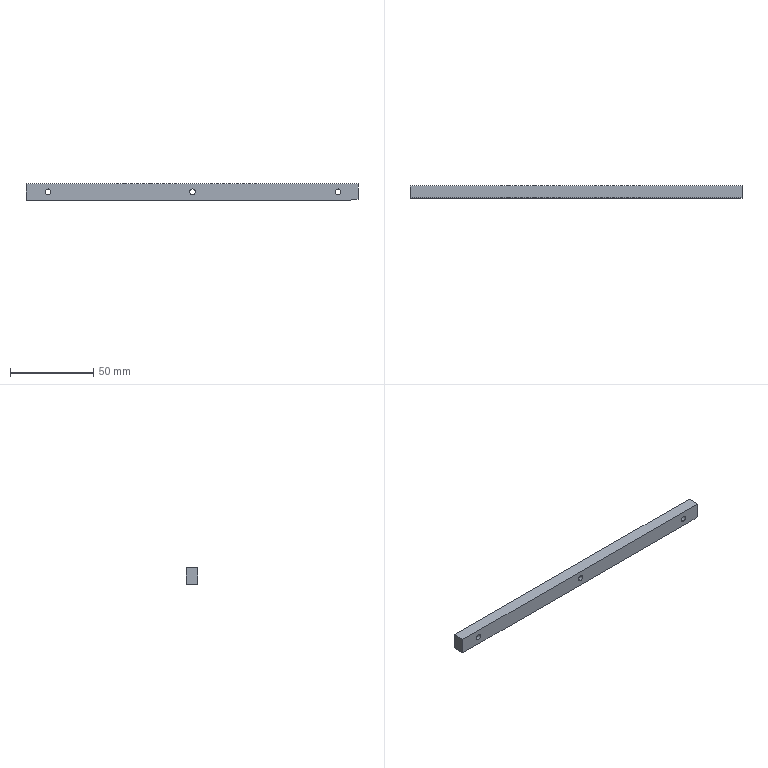Part | NX | 1 solid | 22 faces | box 199.5 x 7.2 x 9.8 mm | volume 13598 mm3 | cylinder 12 | plane 10 | commonest cylinder face diameters 3.5 x6 6 x6
STEP:
#1=CARTESIAN_POINT('',(659.5,215.9,-18.4));
#2=VERTEX_POINT('',#1);
#3=CARTESIAN_POINT('',(659.5,215.9,-27.763));
#4=VERTEX_POINT('',#3);
#5=CARTESIAN_POINT('',(659.5,215.9,-24.851));
#6=DIRECTION('',(0.,0.,-1.));
#7=VECTOR('',#6,1000.);
#8=LINE('',#5,#7);
#9=EDGE_CURVE('',#2,#4,#8,.T.);
#10=ORIENTED_EDGE('',*,*,#9,.T.);
#11=CARTESIAN_POINT('',(654.5,215.9,-28.2));
#12=VERTEX_POINT('',#11);
#13=CARTESIAN_POINT('',(660.,215.9,-27.719));
#14=DIRECTION('',(-0.9962,0.,-0.08716));
#15=VECTOR('',#14,1000.);
#16=LINE('',#13,#15);
#17=EDGE_CURVE('',#4,#12,#16,.T.);
#18=ORIENTED_EDGE('',*,*,#17,.T.);
#19=CARTESIAN_POINT('',(460.,215.9,-28.2));
#20=VERTEX_POINT('',#19);
#21=CARTESIAN_POINT('',(660.,215.9,-28.2));
#22=DIRECTION('',(1.,0.,0.));
#23=VECTOR('',#22,1000.);
#24=LINE('',#21,#23);
#25=EDGE_CURVE('',#20,#12,#24,.T.);
#26=ORIENTED_EDGE('',*,*,#25,.F.);
#27=CARTESIAN_POINT('',(460.,215.9,-18.4));
#28=VERTEX_POINT('',#27);
#29=CARTESIAN_POINT('',(460.,215.9,-24.851));
#30=DIRECTION('',(0.,0.,1.));
#31=VECTOR('',#30,1000.);
#32=LINE('',#29,#31);
#33=EDGE_CURVE('',#20,#28,#32,.T.);
#34=ORIENTED_EDGE('',*,*,#33,.T.);
#35=CARTESIAN_POINT('',(660.,215.9,-18.4));
#36=DIRECTION('',(1.,0.,0.));
#37=VECTOR('',#36,1000.);
#38=LINE('',#35,#37);
#39=EDGE_CURVE('',#28,#2,#38,.T.);
#40=ORIENTED_EDGE('',*,*,#39,.T.);
#41=EDGE_LOOP('',(#10,#18,#26,#34,#40));
#42=FACE_BOUND('',#41,.T.);
#43=CARTESIAN_POINT('',(647.5,215.9,-20.2));
#44=VERTEX_POINT('',#43);
#45=CARTESIAN_POINT('',(647.5,215.9,-26.2));
#46=VERTEX_POINT('',#45);
#47=CARTESIAN_POINT('',(647.5,215.9,-23.2));
#48=DIRECTION('',(0.,1.,0.));
#49=DIRECTION('',(0.,0.,-1.));
#50=AXIS2_PLACEMENT_3D('',#47,#48,#49);
#51=CIRCLE('',#50,3.);
#52=EDGE_CURVE('',#44,#46,#51,.T.);
#53=ORIENTED_EDGE('',*,*,#52,.F.);
#54=CARTESIAN_POINT('',(647.5,215.9,-23.2));
#55=DIRECTION('',(0.,1.,0.));
#56=DIRECTION('',(0.,0.,-1.));
#57=AXIS2_PLACEMENT_3D('',#54,#55,#56);
#58=CIRCLE('',#57,3.);
#59=EDGE_CURVE('',#46,#44,#58,.T.);
#60=ORIENTED_EDGE('',*,*,#59,.F.);
#61=EDGE_LOOP('',(#53,#60));
#62=FACE_BOUND('',#61,.T.);
#63=CARTESIAN_POINT('',(560.,215.9,-20.2));
#64=VERTEX_POINT('',#63);
#65=CARTESIAN_POINT('',(560.,215.9,-26.2));
#66=VERTEX_POINT('',#65);
#67=CARTESIAN_POINT('',(560.,215.9,-23.2));
#68=DIRECTION('',(0.,1.,0.));
#69=DIRECTION('',(0.,0.,-1.));
#70=AXIS2_PLACEMENT_3D('',#67,#68,#69);
#71=CIRCLE('',#70,3.);
#72=EDGE_CURVE('',#64,#66,#71,.T.);
#73=ORIENTED_EDGE('',*,*,#72,.F.);
#74=CARTESIAN_POINT('',(560.,215.9,-23.2));
#75=DIRECTION('',(0.,1.,0.));
#76=DIRECTION('',(0.,0.,-1.));
#77=AXIS2_PLACEMENT_3D('',#74,#75,#76);
#78=CIRCLE('',#77,3.);
#79=EDGE_CURVE('',#66,#64,#78,.T.);
#80=ORIENTED_EDGE('',*,*,#79,.F.);
#81=EDGE_LOOP('',(#73,#80));
#82=FACE_BOUND('',#81,.T.);
#83=CARTESIAN_POINT('',(473.248,215.9,-20.2));
#84=VERTEX_POINT('',#83);
#85=CARTESIAN_POINT('',(473.248,215.9,-26.2));
#86=VERTEX_POINT('',#85);
#87=CARTESIAN_POINT('',(473.248,215.9,-23.2));
#88=DIRECTION('',(0.,1.,0.));
#89=DIRECTION('',(0.,0.,-1.));
#90=AXIS2_PLACEMENT_3D('',#87,#88,#89);
#91=CIRCLE('',#90,3.);
#92=EDGE_CURVE('',#84,#86,#91,.T.);
#93=ORIENTED_EDGE('',*,*,#92,.F.);
#94=CARTESIAN_POINT('',(473.248,215.9,-23.2));
#95=DIRECTION('',(0.,1.,0.));
#96=DIRECTION('',(0.,0.,-1.));
#97=AXIS2_PLACEMENT_3D('',#94,#95,#96);
#98=CIRCLE('',#97,3.);
#99=EDGE_CURVE('',#86,#84,#98,.T.);
#100=ORIENTED_EDGE('',*,*,#99,.F.);
#101=EDGE_LOOP('',(#93,#100));
#102=FACE_BOUND('',#101,.T.);
#103=CARTESIAN_POINT('',(660.,215.9,-28.2));
#104=DIRECTION('',(0.,1.,0.));
#105=DIRECTION('',(1.,0.,0.));
#106=AXIS2_PLACEMENT_3D('',#103,#104,#105);
#107=PLANE('',#106);
#108=ADVANCED_FACE('',(#42,#62,#82,#102),#107,.T.);
#109=CARTESIAN_POINT('',(654.5,208.7,-28.2));
#110=VERTEX_POINT('',#109);
#111=CARTESIAN_POINT('',(654.5,212.3,-28.2));
#112=DIRECTION('',(0.,-1.,0.));
#113=VECTOR('',#112,1000.);
#114=LINE('',#111,#113);
#115=EDGE_CURVE('',#12,#110,#114,.T.);
#116=ORIENTED_EDGE('',*,*,#115,.T.);
#117=CARTESIAN_POINT('',(460.,208.7,-28.2));
#118=VERTEX_POINT('',#117);
#119=CARTESIAN_POINT('',(660.,208.7,-28.2));
#120=DIRECTION('',(-1.,0.,0.));
#121=VECTOR('',#120,1000.);
#122=LINE('',#119,#121);
#123=EDGE_CURVE('',#110,#118,#122,.T.);
#124=ORIENTED_EDGE('',*,*,#123,.T.);
#125=CARTESIAN_POINT('',(460.,203.631,-28.2));
#126=DIRECTION('',(0.,-1.,0.));
#127=VECTOR('',#126,1000.);
#128=LINE('',#125,#127);
#129=EDGE_CURVE('',#20,#118,#128,.T.);
#130=ORIENTED_EDGE('',*,*,#129,.F.);
#131=ORIENTED_EDGE('',*,*,#25,.T.);
#132=EDGE_LOOP('',(#116,#124,#130,#131));
#133=FACE_BOUND('',#132,.T.);
#134=CARTESIAN_POINT('',(660.,208.7,-28.2));
#135=DIRECTION('',(0.,0.,-1.));
#136=DIRECTION('',(-1.,0.,0.));
#137=AXIS2_PLACEMENT_3D('',#134,#135,#136);
#138=PLANE('',#137);
#139=ADVANCED_FACE('',(#133),#138,.T.);
#140=CARTESIAN_POINT('',(659.5,208.7,-27.763));
#141=VERTEX_POINT('',#140);
#142=CARTESIAN_POINT('',(659.5,208.7,-18.4));
#143=VERTEX_POINT('',#142);
#144=CARTESIAN_POINT('',(659.5,208.7,-24.851));
#145=DIRECTION('',(0.,0.,1.));
#146=VECTOR('',#145,1000.);
#147=LINE('',#144,#146);
#148=EDGE_CURVE('',#141,#143,#147,.T.);
#149=ORIENTED_EDGE('',*,*,#148,.T.);
#150=CARTESIAN_POINT('',(460.,208.7,-18.4));
#151=VERTEX_POINT('',#150);
#152=CARTESIAN_POINT('',(660.,208.7,-18.4));
#153=DIRECTION('',(-1.,0.,0.));
#154=VECTOR('',#153,1000.);
#155=LINE('',#152,#154);
#156=EDGE_CURVE('',#143,#151,#155,.T.);
#157=ORIENTED_EDGE('',*,*,#156,.T.);
#158=CARTESIAN_POINT('',(460.,208.7,-24.851));
#159=DIRECTION('',(0.,0.,1.));
#160=VECTOR('',#159,1000.);
#161=LINE('',#158,#160);
#162=EDGE_CURVE('',#118,#151,#161,.T.);
#163=ORIENTED_EDGE('',*,*,#162,.F.);
#164=ORIENTED_EDGE('',*,*,#123,.F.);
#165=CARTESIAN_POINT('',(660.,208.7,-27.719));
#166=DIRECTION('',(0.9962,0.,0.08716));
#167=VECTOR('',#166,1000.);
#168=LINE('',#165,#167);
#169=EDGE_CURVE('',#110,#141,#168,.T.);
#170=ORIENTED_EDGE('',*,*,#169,.T.);
#171=EDGE_LOOP('',(#149,#157,#163,#164,#170));
#172=FACE_BOUND('',#171,.T.);
#173=CARTESIAN_POINT('',(473.248,208.7,-21.45));
#174=VERTEX_POINT('',#173);
#175=CARTESIAN_POINT('',(473.248,208.7,-24.95));
#176=VERTEX_POINT('',#175);
#177=CARTESIAN_POINT('',(473.248,208.7,-23.2));
#178=DIRECTION('',(0.,1.,0.));
#179=DIRECTION('',(0.,0.,-1.));
#180=AXIS2_PLACEMENT_3D('',#177,#178,#179);
#181=CIRCLE('',#180,1.75);
#182=EDGE_CURVE('',#174,#176,#181,.T.);
#183=ORIENTED_EDGE('',*,*,#182,.T.);
#184=CARTESIAN_POINT('',(473.248,208.7,-23.2));
#185=DIRECTION('',(0.,1.,0.));
#186=DIRECTION('',(0.,0.,-1.));
#187=AXIS2_PLACEMENT_3D('',#184,#185,#186);
#188=CIRCLE('',#187,1.75);
#189=EDGE_CURVE('',#176,#174,#188,.T.);
#190=ORIENTED_EDGE('',*,*,#189,.T.);
#191=EDGE_LOOP('',(#183,#190));
#192=FACE_BOUND('',#191,.T.);
#193=CARTESIAN_POINT('',(647.5,208.7,-24.95));
#194=VERTEX_POINT('',#193);
#195=CARTESIAN_POINT('',(647.5,208.7,-21.45));
#196=VERTEX_POINT('',#195);
#197=CARTESIAN_POINT('',(647.5,208.7,-23.2));
#198=DIRECTION('',(0.,1.,0.));
#199=DIRECTION('',(0.,0.,-1.));
#200=AXIS2_PLACEMENT_3D('',#197,#198,#199);
#201=CIRCLE('',#200,1.75);
#202=EDGE_CURVE('',#194,#196,#201,.T.);
#203=ORIENTED_EDGE('',*,*,#202,.T.);
#204=CARTESIAN_POINT('',(647.5,208.7,-23.2));
#205=DIRECTION('',(0.,1.,0.));
#206=DIRECTION('',(0.,0.,-1.));
#207=AXIS2_PLACEMENT_3D('',#204,#205,#206);
#208=CIRCLE('',#207,1.75);
#209=EDGE_CURVE('',#196,#194,#208,.T.);
#210=ORIENTED_EDGE('',*,*,#209,.T.);
#211=EDGE_LOOP('',(#203,#210));
#212=FACE_BOUND('',#211,.T.);
#213=CARTESIAN_POINT('',(560.,208.7,-24.95));
#214=VERTEX_POINT('',#213);
#215=CARTESIAN_POINT('',(560.,208.7,-21.45));
#216=VERTEX_POINT('',#215);
#217=CARTESIAN_POINT('',(560.,208.7,-23.2));
#218=DIRECTION('',(0.,1.,0.));
#219=DIRECTION('',(0.,0.,-1.));
#220=AXIS2_PLACEMENT_3D('',#217,#218,#219);
#221=CIRCLE('',#220,1.75);
#222=EDGE_CURVE('',#214,#216,#221,.T.);
#223=ORIENTED_EDGE('',*,*,#222,.T.);
#224=CARTESIAN_POINT('',(560.,208.7,-23.2));
#225=DIRECTION('',(0.,1.,0.));
#226=DIRECTION('',(0.,0.,-1.));
#227=AXIS2_PLACEMENT_3D('',#224,#225,#226);
#228=CIRCLE('',#227,1.75);
#229=EDGE_CURVE('',#216,#214,#228,.T.);
#230=ORIENTED_EDGE('',*,*,#229,.T.);
#231=EDGE_LOOP('',(#223,#230));
#232=FACE_BOUND('',#231,.T.);
#233=CARTESIAN_POINT('',(660.,208.7,-18.2));
#234=DIRECTION('',(0.,-1.,0.));
#235=DIRECTION('',(-1.,0.,0.));
#236=AXIS2_PLACEMENT_3D('',#233,#234,#235);
#237=PLANE('',#236);
#238=ADVANCED_FACE('',(#172,#192,#212,#232),#237,.T.);
#239=CARTESIAN_POINT('',(659.5,203.631,-18.4));
#240=DIRECTION('',(0.,1.,0.));
#241=VECTOR('',#240,1000.);
#242=LINE('',#239,#241);
#243=EDGE_CURVE('',#143,#2,#242,.T.);
#244=ORIENTED_EDGE('',*,*,#243,.T.);
#245=ORIENTED_EDGE('',*,*,#39,.F.);
#246=CARTESIAN_POINT('',(460.,203.631,-18.4));
#247=DIRECTION('',(0.,-1.,0.));
#248=VECTOR('',#247,1000.);
#249=LINE('',#246,#248);
#250=EDGE_CURVE('',#28,#151,#249,.T.);
#251=ORIENTED_EDGE('',*,*,#250,.T.);
#252=ORIENTED_EDGE('',*,*,#156,.F.);
#253=EDGE_LOOP('',(#244,#245,#251,#252));
#254=FACE_BOUND('',#253,.T.);
#255=CARTESIAN_POINT('',(660.,214.7,-18.4));
#256=DIRECTION('',(0.,0.,1.));
#257=DIRECTION('',(1.,0.,0.));
#258=AXIS2_PLACEMENT_3D('',#255,#256,#257);
#259=PLANE('',#258);
#260=ADVANCED_FACE('',(#254),#259,.T.);
#261=ORIENTED_EDGE('',*,*,#202,.F.);
#262=CARTESIAN_POINT('',(647.5,211.2,-24.95));
#263=VERTEX_POINT('',#262);
#264=CARTESIAN_POINT('',(647.5,214.7,-24.95));
#265=DIRECTION('',(0.,1.,0.));
#266=VECTOR('',#265,1000.);
#267=LINE('',#264,#266);
#268=EDGE_CURVE('',#263,#194,#267,.F.);
#269=ORIENTED_EDGE('',*,*,#268,.F.);
#270=CARTESIAN_POINT('',(647.5,211.2,-21.45));
#271=VERTEX_POINT('',#270);
#272=CARTESIAN_POINT('',(647.5,211.2,-23.2));
#273=DIRECTION('',(0.,1.,0.));
#274=DIRECTION('',(0.,0.,-1.));
#275=AXIS2_PLACEMENT_3D('',#272,#273,#274);
#276=CIRCLE('',#275,1.75);
#277=EDGE_CURVE('',#263,#271,#276,.T.);
#278=ORIENTED_EDGE('',*,*,#277,.T.);
#279=CARTESIAN_POINT('',(647.5,214.7,-21.45));
#280=DIRECTION('',(0.,1.,0.));
#281=VECTOR('',#280,1000.);
#282=LINE('',#279,#281);
#283=EDGE_CURVE('',#271,#196,#282,.F.);
#284=ORIENTED_EDGE('',*,*,#283,.T.);
#285=EDGE_LOOP('',(#261,#269,#278,#284));
#286=FACE_BOUND('',#285,.T.);
#287=CARTESIAN_POINT('',(647.5,214.7,-23.2));
#288=DIRECTION('',(0.,1.,0.));
#289=DIRECTION('',(0.,0.,-1.));
#290=AXIS2_PLACEMENT_3D('',#287,#288,#289);
#291=CYLINDRICAL_SURFACE('',#290,1.75);
#292=ADVANCED_FACE('',(#286),#291,.F.);
#293=CARTESIAN_POINT('',(647.5,211.2,-20.2));
#294=VERTEX_POINT('',#293);
#295=CARTESIAN_POINT('',(647.5,211.2,-26.2));
#296=VERTEX_POINT('',#295);
#297=CARTESIAN_POINT('',(647.5,211.2,-23.2));
#298=DIRECTION('',(0.,1.,0.));
#299=DIRECTION('',(0.,0.,-1.));
#300=AXIS2_PLACEMENT_3D('',#297,#298,#299);
#301=CIRCLE('',#300,3.);
#302=EDGE_CURVE('',#294,#296,#301,.T.);
#303=ORIENTED_EDGE('',*,*,#302,.T.);
#304=CARTESIAN_POINT('',(647.5,211.2,-23.2));
#305=DIRECTION('',(0.,1.,0.));
#306=DIRECTION('',(0.,0.,-1.));
#307=AXIS2_PLACEMENT_3D('',#304,#305,#306);
#308=CIRCLE('',#307,3.);
#309=EDGE_CURVE('',#296,#294,#308,.T.);
#310=ORIENTED_EDGE('',*,*,#309,.T.);
#311=EDGE_LOOP('',(#303,#310));
#312=FACE_BOUND('',#311,.T.);
#313=CARTESIAN_POINT('',(647.5,211.2,-23.2));
#314=DIRECTION('',(0.,1.,0.));
#315=DIRECTION('',(0.,0.,-1.));
#316=AXIS2_PLACEMENT_3D('',#313,#314,#315);
#317=CIRCLE('',#316,1.75);
#318=EDGE_CURVE('',#271,#263,#317,.T.);
#319=ORIENTED_EDGE('',*,*,#318,.F.);
#320=ORIENTED_EDGE('',*,*,#277,.F.);
#321=EDGE_LOOP('',(#319,#320));
#322=FACE_BOUND('',#321,.T.);
#323=CARTESIAN_POINT('',(647.5,211.2,-23.2));
#324=DIRECTION('',(0.,1.,0.));
#325=DIRECTION('',(1.,0.,0.));
#326=AXIS2_PLACEMENT_3D('',#323,#324,#325);
#327=PLANE('',#326);
#328=ADVANCED_FACE('',(#312,#322),#327,.T.);
#329=ORIENTED_EDGE('',*,*,#52,.T.);
#330=CARTESIAN_POINT('',(647.5,214.7,-26.2));
#331=DIRECTION('',(0.,1.,0.));
#332=VECTOR('',#331,1000.);
#333=LINE('',#330,#332);
#334=EDGE_CURVE('',#296,#46,#333,.T.);
#335=ORIENTED_EDGE('',*,*,#334,.F.);
#336=ORIENTED_EDGE('',*,*,#302,.F.);
#337=CARTESIAN_POINT('',(647.5,214.7,-20.2));
#338=DIRECTION('',(0.,1.,0.));
#339=VECTOR('',#338,1000.);
#340=LINE('',#337,#339);
#341=EDGE_CURVE('',#294,#44,#340,.T.);
#342=ORIENTED_EDGE('',*,*,#341,.T.);
#343=EDGE_LOOP('',(#329,#335,#336,#342));
#344=FACE_BOUND('',#343,.T.);
#345=CARTESIAN_POINT('',(647.5,214.7,-23.2));
#346=DIRECTION('',(0.,1.,0.));
#347=DIRECTION('',(0.,0.,-1.));
#348=AXIS2_PLACEMENT_3D('',#345,#346,#347);
#349=CYLINDRICAL_SURFACE('',#348,3.);
#350=ADVANCED_FACE('',(#344),#349,.F.);
#351=ORIENTED_EDGE('',*,*,#72,.T.);
#352=CARTESIAN_POINT('',(560.,211.2,-26.2));
#353=VERTEX_POINT('',#352);
#354=CARTESIAN_POINT('',(560.,214.7,-26.2));
#355=DIRECTION('',(0.,1.,0.));
#356=VECTOR('',#355,1000.);
#357=LINE('',#354,#356);
#358=EDGE_CURVE('',#353,#66,#357,.T.);
#359=ORIENTED_EDGE('',*,*,#358,.F.);
#360=CARTESIAN_POINT('',(560.,211.2,-20.2));
#361=VERTEX_POINT('',#360);
#362=CARTESIAN_POINT('',(560.,211.2,-23.2));
#363=DIRECTION('',(0.,1.,0.));
#364=DIRECTION('',(0.,0.,-1.));
#365=AXIS2_PLACEMENT_3D('',#362,#363,#364);
#366=CIRCLE('',#365,3.);
#367=EDGE_CURVE('',#361,#353,#366,.T.);
#368=ORIENTED_EDGE('',*,*,#367,.F.);
#369=CARTESIAN_POINT('',(560.,214.7,-20.2));
#370=DIRECTION('',(0.,1.,0.));
#371=VECTOR('',#370,1000.);
#372=LINE('',#369,#371);
#373=EDGE_CURVE('',#361,#64,#372,.T.);
#374=ORIENTED_EDGE('',*,*,#373,.T.);
#375=EDGE_LOOP('',(#351,#359,#368,#374));
#376=FACE_BOUND('',#375,.T.);
#377=CARTESIAN_POINT('',(560.,214.7,-23.2));
#378=DIRECTION('',(0.,1.,0.));
#379=DIRECTION('',(0.,0.,-1.));
#380=AXIS2_PLACEMENT_3D('',#377,#378,#379);
#381=CYLINDRICAL_SURFACE('',#380,3.);
#382=ADVANCED_FACE('',(#376),#381,.F.);
#383=ORIENTED_EDGE('',*,*,#367,.T.);
#384=CARTESIAN_POINT('',(560.,211.2,-23.2));
#385=DIRECTION('',(0.,1.,0.));
#386=DIRECTION('',(0.,0.,-1.));
#387=AXIS2_PLACEMENT_3D('',#384,#385,#386);
#388=CIRCLE('',#387,3.);
#389=EDGE_CURVE('',#353,#361,#388,.T.);
#390=ORIENTED_EDGE('',*,*,#389,.T.);
#391=EDGE_LOOP('',(#383,#390));
#392=FACE_BOUND('',#391,.T.);
#393=CARTESIAN_POINT('',(560.,211.2,-24.95));
#394=VERTEX_POINT('',#393);
#395=CARTESIAN_POINT('',(560.,211.2,-21.45));
#396=VERTEX_POINT('',#395);
#397=CARTESIAN_POINT('',(560.,211.2,-23.2));
#398=DIRECTION('',(0.,1.,0.));
#399=DIRECTION('',(0.,0.,-1.));
#400=AXIS2_PLACEMENT_3D('',#397,#398,#399);
#401=CIRCLE('',#400,1.75);
#402=EDGE_CURVE('',#394,#396,#401,.T.);
#403=ORIENTED_EDGE('',*,*,#402,.F.);
#404=CARTESIAN_POINT('',(560.,211.2,-23.2));
#405=DIRECTION('',(0.,1.,0.));
#406=DIRECTION('',(0.,0.,-1.));
#407=AXIS2_PLACEMENT_3D('',#404,#405,#406);
#408=CIRCLE('',#407,1.75);
#409=EDGE_CURVE('',#396,#394,#408,.T.);
#410=ORIENTED_EDGE('',*,*,#409,.F.);
#411=EDGE_LOOP('',(#403,#410));
#412=FACE_BOUND('',#411,.T.);
#413=CARTESIAN_POINT('',(560.,211.2,-23.2));
#414=DIRECTION('',(0.,1.,0.));
#415=DIRECTION('',(1.,0.,0.));
#416=AXIS2_PLACEMENT_3D('',#413,#414,#415);
#417=PLANE('',#416);
#418=ADVANCED_FACE('',(#392,#412),#417,.T.);
#419=ORIENTED_EDGE('',*,*,#402,.T.);
#420=CARTESIAN_POINT('',(560.,214.7,-21.45));
#421=DIRECTION('',(0.,1.,0.));
#422=VECTOR('',#421,1000.);
#423=LINE('',#420,#422);
#424=EDGE_CURVE('',#396,#216,#423,.F.);
#425=ORIENTED_EDGE('',*,*,#424,.T.);
#426=ORIENTED_EDGE('',*,*,#222,.F.);
#427=CARTESIAN_POINT('',(560.,214.7,-24.95));
#428=DIRECTION('',(0.,1.,0.));
#429=VECTOR('',#428,1000.);
#430=LINE('',#427,#429);
#431=EDGE_CURVE('',#394,#214,#430,.F.);
#432=ORIENTED_EDGE('',*,*,#431,.F.);
#433=EDGE_LOOP('',(#419,#425,#426,#432));
#434=FACE_BOUND('',#433,.T.);
#435=CARTESIAN_POINT('',(560.,214.7,-23.2));
#436=DIRECTION('',(0.,1.,0.));
#437=DIRECTION('',(0.,0.,-1.));
#438=AXIS2_PLACEMENT_3D('',#435,#436,#437);
#439=CYLINDRICAL_SURFACE('',#438,1.75);
#440=ADVANCED_FACE('',(#434),#439,.F.);
#441=CARTESIAN_POINT('',(473.248,211.2,-26.2));
#442=VERTEX_POINT('',#441);
#443=CARTESIAN_POINT('',(473.248,211.2,-20.2));
#444=VERTEX_POINT('',#443);
#445=CARTESIAN_POINT('',(473.248,211.2,-23.2));
#446=DIRECTION('',(0.,1.,0.));
#447=DIRECTION('',(0.,0.,-1.));
#448=AXIS2_PLACEMENT_3D('',#445,#446,#447);
#449=CIRCLE('',#448,3.);
#450=EDGE_CURVE('',#442,#444,#449,.T.);
#451=ORIENTED_EDGE('',*,*,#450,.F.);
#452=CARTESIAN_POINT('',(473.248,214.7,-26.2));
#453=DIRECTION('',(0.,1.,0.));
#454=VECTOR('',#453,1000.);
#455=LINE('',#452,#454);
#456=EDGE_CURVE('',#86,#442,#455,.F.);
#457=ORIENTED_EDGE('',*,*,#456,.F.);
#458=ORIENTED_EDGE('',*,*,#99,.T.);
#459=CARTESIAN_POINT('',(473.248,214.7,-20.2));
#460=DIRECTION('',(0.,1.,0.));
#461=VECTOR('',#460,1000.);
#462=LINE('',#459,#461);
#463=EDGE_CURVE('',#84,#444,#462,.F.);
#464=ORIENTED_EDGE('',*,*,#463,.T.);
#465=EDGE_LOOP('',(#451,#457,#458,#464));
#466=FACE_BOUND('',#465,.T.);
#467=CARTESIAN_POINT('',(473.248,214.7,-23.2));
#468=DIRECTION('',(0.,1.,0.));
#469=DIRECTION('',(0.,0.,-1.));
#470=AXIS2_PLACEMENT_3D('',#467,#468,#469);
#471=CYLINDRICAL_SURFACE('',#470,3.);
#472=ADVANCED_FACE('',(#466),#471,.F.);
#473=ORIENTED_EDGE('',*,*,#450,.T.);
#474=CARTESIAN_POINT('',(473.248,211.2,-23.2));
#475=DIRECTION('',(0.,1.,0.));
#476=DIRECTION('',(0.,0.,-1.));
#477=AXIS2_PLACEMENT_3D('',#474,#475,#476);
#478=CIRCLE('',#477,3.);
#479=EDGE_CURVE('',#444,#442,#478,.T.);
#480=ORIENTED_EDGE('',*,*,#479,.T.);
#481=EDGE_LOOP('',(#473,#480));
#482=FACE_BOUND('',#481,.T.);
#483=CARTESIAN_POINT('',(473.248,211.2,-21.45));
#484=VERTEX_POINT('',#483);
#485=CARTESIAN_POINT('',(473.248,211.2,-24.95));
#486=VERTEX_POINT('',#485);
#487=CARTESIAN_POINT('',(473.248,211.2,-23.2));
#488=DIRECTION('',(0.,1.,0.));
#489=DIRECTION('',(0.,0.,-1.));
#490=AXIS2_PLACEMENT_3D('',#487,#488,#489);
#491=CIRCLE('',#490,1.75);
#492=EDGE_CURVE('',#484,#486,#491,.T.);
#493=ORIENTED_EDGE('',*,*,#492,.F.);
#494=CARTESIAN_POINT('',(473.248,211.2,-23.2));
#495=DIRECTION('',(0.,1.,0.));
#496=DIRECTION('',(0.,0.,-1.));
#497=AXIS2_PLACEMENT_3D('',#494,#495,#496);
#498=CIRCLE('',#497,1.75);
#499=EDGE_CURVE('',#486,#484,#498,.T.);
#500=ORIENTED_EDGE('',*,*,#499,.F.);
#501=EDGE_LOOP('',(#493,#500));
#502=FACE_BOUND('',#501,.T.);
#503=CARTESIAN_POINT('',(473.248,211.2,-23.2));
#504=DIRECTION('',(0.,1.,0.));
#505=DIRECTION('',(1.,0.,0.));
#506=AXIS2_PLACEMENT_3D('',#503,#504,#505);
#507=PLANE('',#506);
#508=ADVANCED_FACE('',(#482,#502),#507,.T.);
#509=ORIENTED_EDGE('',*,*,#182,.F.);
#510=CARTESIAN_POINT('',(473.248,214.7,-21.45));
#511=DIRECTION('',(0.,1.,0.));
#512=VECTOR('',#511,1000.);
#513=LINE('',#510,#512);
#514=EDGE_CURVE('',#484,#174,#513,.F.);
#515=ORIENTED_EDGE('',*,*,#514,.F.);
#516=ORIENTED_EDGE('',*,*,#492,.T.);
#517=CARTESIAN_POINT('',(473.248,214.7,-24.95));
#518=DIRECTION('',(0.,1.,0.));
#519=VECTOR('',#518,1000.);
#520=LINE('',#517,#519);
#521=EDGE_CURVE('',#486,#176,#520,.F.);
#522=ORIENTED_EDGE('',*,*,#521,.T.);
#523=EDGE_LOOP('',(#509,#515,#516,#522));
#524=FACE_BOUND('',#523,.T.);
#525=CARTESIAN_POINT('',(473.248,214.7,-23.2));
#526=DIRECTION('',(0.,1.,0.));
#527=DIRECTION('',(0.,0.,-1.));
#528=AXIS2_PLACEMENT_3D('',#525,#526,#527);
#529=CYLINDRICAL_SURFACE('',#528,1.75);
#530=ADVANCED_FACE('',(#524),#529,.F.);
#531=CARTESIAN_POINT('',(659.5,212.3,-27.763));
#532=DIRECTION('',(0.,-1.,0.));
#533=VECTOR('',#532,1000.);
#534=LINE('',#531,#533);
#535=EDGE_CURVE('',#4,#141,#534,.T.);
#536=ORIENTED_EDGE('',*,*,#535,.T.);
#537=ORIENTED_EDGE('',*,*,#169,.F.);
#538=ORIENTED_EDGE('',*,*,#115,.F.);
#539=ORIENTED_EDGE('',*,*,#17,.F.);
#540=EDGE_LOOP('',(#536,#537,#538,#539));
#541=FACE_BOUND('',#540,.T.);
#542=CARTESIAN_POINT('',(657.,212.3,-27.981));
#543=DIRECTION('',(-0.08716,0.,0.9962));
#544=DIRECTION('',(0.,1.,0.));
#545=AXIS2_PLACEMENT_3D('',#542,#543,#544);
#546=PLANE('',#545);
#547=ADVANCED_FACE('',(#541),#546,.F.);
#548=ORIENTED_EDGE('',*,*,#250,.F.);
#549=ORIENTED_EDGE('',*,*,#33,.F.);
#550=ORIENTED_EDGE('',*,*,#129,.T.);
#551=ORIENTED_EDGE('',*,*,#162,.T.);
#552=EDGE_LOOP('',(#548,#549,#550,#551));
#553=FACE_BOUND('',#552,.T.);
#554=CARTESIAN_POINT('',(460.,203.631,-24.851));
#555=DIRECTION('',(1.,0.,0.));
#556=DIRECTION('',(0.,-1.,0.));
#557=AXIS2_PLACEMENT_3D('',#554,#555,#556);
#558=PLANE('',#557);
#559=ADVANCED_FACE('',(#553),#558,.F.);
#560=ORIENTED_EDGE('',*,*,#535,.F.);
#561=ORIENTED_EDGE('',*,*,#9,.F.);
#562=ORIENTED_EDGE('',*,*,#243,.F.);
#563=ORIENTED_EDGE('',*,*,#148,.F.);
#564=EDGE_LOOP('',(#560,#561,#562,#563));
#565=FACE_BOUND('',#564,.T.);
#566=CARTESIAN_POINT('',(659.5,203.631,-24.851));
#567=DIRECTION('',(1.,0.,0.));
#568=DIRECTION('',(0.,-1.,0.));
#569=AXIS2_PLACEMENT_3D('',#566,#567,#568);
#570=PLANE('',#569);
#571=ADVANCED_FACE('',(#565),#570,.T.);
#572=ORIENTED_EDGE('',*,*,#521,.F.);
#573=ORIENTED_EDGE('',*,*,#499,.T.);
#574=ORIENTED_EDGE('',*,*,#514,.T.);
#575=ORIENTED_EDGE('',*,*,#189,.F.);
#576=EDGE_LOOP('',(#572,#573,#574,#575));
#577=FACE_BOUND('',#576,.T.);
#578=CARTESIAN_POINT('',(473.248,214.7,-23.2));
#579=DIRECTION('',(0.,1.,0.));
#580=DIRECTION('',(0.,0.,-1.));
#581=AXIS2_PLACEMENT_3D('',#578,#579,#580);
#582=CYLINDRICAL_SURFACE('',#581,1.75);
#583=ADVANCED_FACE('',(#577),#582,.F.);
#584=ORIENTED_EDGE('',*,*,#373,.F.);
#585=ORIENTED_EDGE('',*,*,#389,.F.);
#586=ORIENTED_EDGE('',*,*,#358,.T.);
#587=ORIENTED_EDGE('',*,*,#79,.T.);
#588=EDGE_LOOP('',(#584,#585,#586,#587));
#589=FACE_BOUND('',#588,.T.);
#590=CARTESIAN_POINT('',(560.,214.7,-23.2));
#591=DIRECTION('',(0.,1.,0.));
#592=DIRECTION('',(0.,0.,-1.));
#593=AXIS2_PLACEMENT_3D('',#590,#591,#592);
#594=CYLINDRICAL_SURFACE('',#593,3.);
#595=ADVANCED_FACE('',(#589),#594,.F.);
#596=ORIENTED_EDGE('',*,*,#318,.T.);
#597=ORIENTED_EDGE('',*,*,#268,.T.);
#598=ORIENTED_EDGE('',*,*,#209,.F.);
#599=ORIENTED_EDGE('',*,*,#283,.F.);
#600=EDGE_LOOP('',(#596,#597,#598,#599));
#601=FACE_BOUND('',#600,.T.);
#602=CARTESIAN_POINT('',(647.5,214.7,-23.2));
#603=DIRECTION('',(0.,1.,0.));
#604=DIRECTION('',(0.,0.,-1.));
#605=AXIS2_PLACEMENT_3D('',#602,#603,#604);
#606=CYLINDRICAL_SURFACE('',#605,1.75);
#607=ADVANCED_FACE('',(#601),#606,.F.);
#608=ORIENTED_EDGE('',*,*,#431,.T.);
#609=ORIENTED_EDGE('',*,*,#229,.F.);
#610=ORIENTED_EDGE('',*,*,#424,.F.);
#611=ORIENTED_EDGE('',*,*,#409,.T.);
#612=EDGE_LOOP('',(#608,#609,#610,#611));
#613=FACE_BOUND('',#612,.T.);
#614=CARTESIAN_POINT('',(560.,214.7,-23.2));
#615=DIRECTION('',(0.,1.,0.));
#616=DIRECTION('',(0.,0.,-1.));
#617=AXIS2_PLACEMENT_3D('',#614,#615,#616);
#618=CYLINDRICAL_SURFACE('',#617,1.75);
#619=ADVANCED_FACE('',(#613),#618,.F.);
#620=ORIENTED_EDGE('',*,*,#341,.F.);
#621=ORIENTED_EDGE('',*,*,#309,.F.);
#622=ORIENTED_EDGE('',*,*,#334,.T.);
#623=ORIENTED_EDGE('',*,*,#59,.T.);
#624=EDGE_LOOP('',(#620,#621,#622,#623));
#625=FACE_BOUND('',#624,.T.);
#626=CARTESIAN_POINT('',(647.5,214.7,-23.2));
#627=DIRECTION('',(0.,1.,0.));
#628=DIRECTION('',(0.,0.,-1.));
#629=AXIS2_PLACEMENT_3D('',#626,#627,#628);
#630=CYLINDRICAL_SURFACE('',#629,3.);
#631=ADVANCED_FACE('',(#625),#630,.F.);
#632=ORIENTED_EDGE('',*,*,#92,.T.);
#633=ORIENTED_EDGE('',*,*,#456,.T.);
#634=ORIENTED_EDGE('',*,*,#479,.F.);
#635=ORIENTED_EDGE('',*,*,#463,.F.);
#636=EDGE_LOOP('',(#632,#633,#634,#635));
#637=FACE_BOUND('',#636,.T.);
#638=CARTESIAN_POINT('',(473.248,214.7,-23.2));
#639=DIRECTION('',(0.,1.,0.));
#640=DIRECTION('',(0.,0.,-1.));
#641=AXIS2_PLACEMENT_3D('',#638,#639,#640);
#642=CYLINDRICAL_SURFACE('',#641,3.);
#643=ADVANCED_FACE('',(#637),#642,.F.);
#644=CLOSED_SHELL('',(#108,#139,#238,#260,#292,#328,#350,#382,#418,#440,#472,#508,#530,#547,#559,#571,#583,#595,#607,#619,#631,#643));
#645=MANIFOLD_SOLID_BREP('',#644);
#646=(LENGTH_UNIT()NAMED_UNIT(*)SI_UNIT(.MILLI.,.METRE.));
#647=UNCERTAINTY_MEASURE_WITH_UNIT(LENGTH_MEASURE(0.00001),#646,'','');
#648=(NAMED_UNIT(*)PLANE_ANGLE_UNIT()SI_UNIT($,.RADIAN.));
#649=(NAMED_UNIT(*)SI_UNIT($,.STERADIAN.)SOLID_ANGLE_UNIT());
#650=(GEOMETRIC_REPRESENTATION_CONTEXT(3)GLOBAL_UNCERTAINTY_ASSIGNED_CONTEXT((#647))GLOBAL_UNIT_ASSIGNED_CONTEXT((#646,#648,#649))REPRESENTATION_CONTEXT('',''));
#651=ADVANCED_BREP_SHAPE_REPRESENTATION('',(#645),#650);